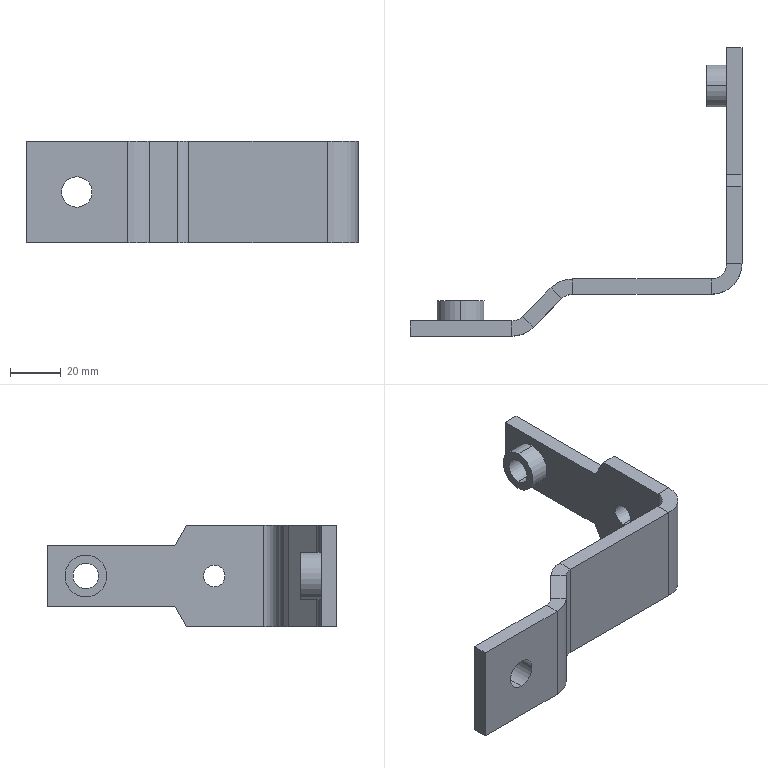Part | STEP file | 64661426 | 1 solid | 46 faces | box 130.6 x 113.5 x 40 mm | volume 49498 mm3 | plane 30 | cylinder 16 | commonest cylinder face diameters 12 x5 24 x3 8.5 x2 10 x2 16.5 x2 18.5 x2